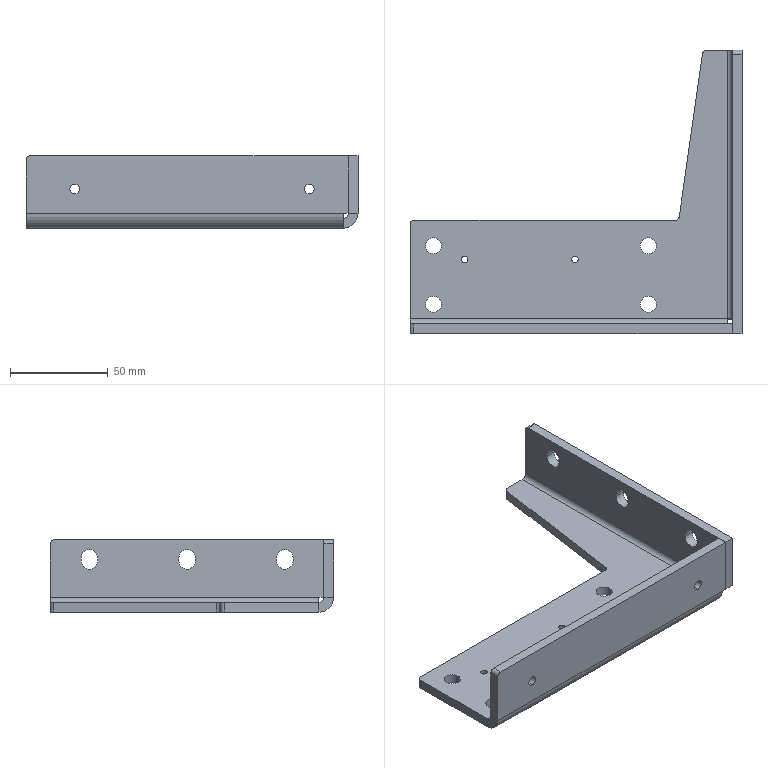Part | STEP file | 1 solid | 62 faces | box 170 x 145 x 37 mm | volume 104270 mm3 | cylinder 34 | plane 28 | commonest cylinder face diameters 8.5 x9 8.2 x8 5 x6 4 x5 3.3 x4 15 x2